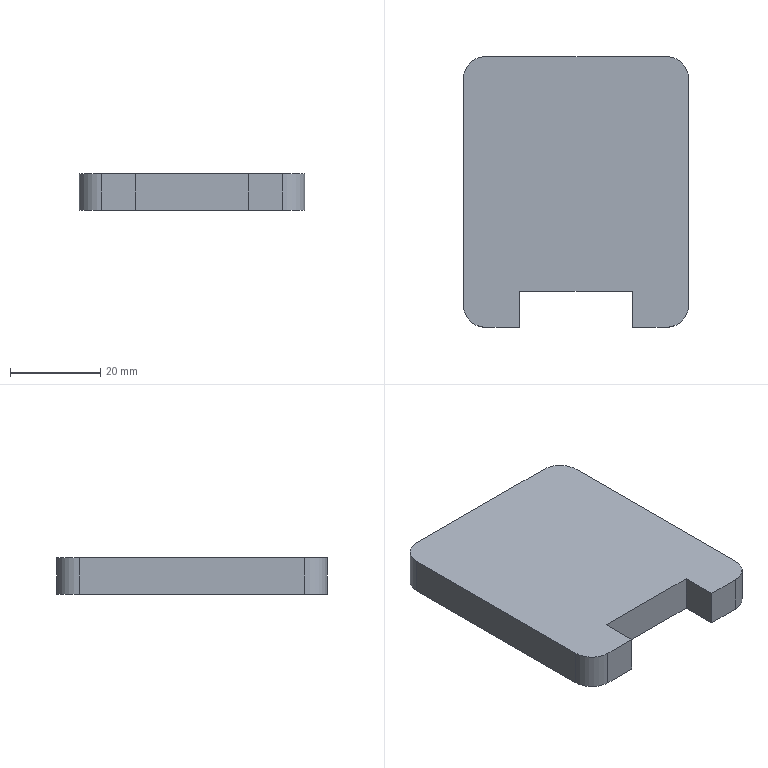Part | SolidWorks | features FlatPattern 1, SMBaseFlange 1, SheetMetal 1 | 1 solid | 14 faces | box 50 x 60 x 8 mm | volume 22228 mm3 | plane 10 | cylinder 4 | commonest cylinder face diameters 10 x4
STEP:
#1=CARTESIAN_POINT('',(-411.372,-6.5,0.));
#2=VERTEX_POINT('',#1);
#3=CARTESIAN_POINT('',(-406.372,-11.5,0.));
#4=VERTEX_POINT('',#3);
#5=CARTESIAN_POINT('',(-406.372,-6.5,0.));
#6=DIRECTION('',(0.,0.,1.));
#7=DIRECTION('',(-1.,0.,0.));
#8=AXIS2_PLACEMENT_3D('',#5,#6,#7);
#9=CIRCLE('',#8,5.);
#10=EDGE_CURVE('',#2,#4,#9,.T.);
#11=ORIENTED_EDGE('',*,*,#10,.F.);
#12=CARTESIAN_POINT('',(-411.372,-6.5,-8.));
#13=VERTEX_POINT('',#12);
#14=CARTESIAN_POINT('',(-411.372,-6.5,-8.));
#15=DIRECTION('',(0.,0.,1.));
#16=VECTOR('',#15,1000.);
#17=LINE('',#14,#16);
#18=EDGE_CURVE('',#13,#2,#17,.T.);
#19=ORIENTED_EDGE('',*,*,#18,.F.);
#20=CARTESIAN_POINT('',(-406.372,-11.5,-8.));
#21=VERTEX_POINT('',#20);
#22=CARTESIAN_POINT('',(-406.372,-6.5,-8.));
#23=DIRECTION('',(0.,0.,1.));
#24=DIRECTION('',(-1.,0.,0.));
#25=AXIS2_PLACEMENT_3D('',#22,#23,#24);
#26=CIRCLE('',#25,5.);
#27=EDGE_CURVE('',#13,#21,#26,.T.);
#28=ORIENTED_EDGE('',*,*,#27,.T.);
#29=CARTESIAN_POINT('',(-406.372,-11.5,-8.));
#30=DIRECTION('',(0.,0.,1.));
#31=VECTOR('',#30,1000.);
#32=LINE('',#29,#31);
#33=EDGE_CURVE('',#21,#4,#32,.T.);
#34=ORIENTED_EDGE('',*,*,#33,.T.);
#35=EDGE_LOOP('',(#11,#19,#28,#34));
#36=FACE_OUTER_BOUND('',#35,.T.);
#37=CARTESIAN_POINT('',(-406.372,-6.5,-8.));
#38=DIRECTION('',(0.,0.,1.));
#39=DIRECTION('',(1.,0.,0.));
#40=AXIS2_PLACEMENT_3D('',#37,#38,#39);
#41=CYLINDRICAL_SURFACE('',#40,5.);
#42=ADVANCED_FACE('',(#36),#41,.T.);
#43=CARTESIAN_POINT('',(-411.372,43.5,0.));
#44=VERTEX_POINT('',#43);
#45=CARTESIAN_POINT('',(-411.372,-6.5,0.));
#46=DIRECTION('',(0.,-1.,0.));
#47=VECTOR('',#46,1000.);
#48=LINE('',#45,#47);
#49=EDGE_CURVE('',#44,#2,#48,.T.);
#50=ORIENTED_EDGE('',*,*,#49,.F.);
#51=CARTESIAN_POINT('',(-411.372,43.5,-8.));
#52=VERTEX_POINT('',#51);
#53=CARTESIAN_POINT('',(-411.372,43.5,-8.));
#54=DIRECTION('',(0.,0.,1.));
#55=VECTOR('',#54,1000.);
#56=LINE('',#53,#55);
#57=EDGE_CURVE('',#52,#44,#56,.T.);
#58=ORIENTED_EDGE('',*,*,#57,.F.);
#59=CARTESIAN_POINT('',(-411.372,-6.5,-8.));
#60=DIRECTION('',(0.,-1.,0.));
#61=VECTOR('',#60,1000.);
#62=LINE('',#59,#61);
#63=EDGE_CURVE('',#52,#13,#62,.T.);
#64=ORIENTED_EDGE('',*,*,#63,.T.);
#65=ORIENTED_EDGE('',*,*,#18,.T.);
#66=EDGE_LOOP('',(#50,#58,#64,#65));
#67=FACE_OUTER_BOUND('',#66,.T.);
#68=CARTESIAN_POINT('',(-411.372,-6.5,-8.));
#69=DIRECTION('',(-1.,0.,0.));
#70=DIRECTION('',(0.,0.,1.));
#71=AXIS2_PLACEMENT_3D('',#68,#69,#70);
#72=PLANE('',#71);
#73=ADVANCED_FACE('',(#67),#72,.T.);
#74=CARTESIAN_POINT('',(-406.372,48.5,0.));
#75=VERTEX_POINT('',#74);
#76=CARTESIAN_POINT('',(-406.372,43.5,0.));
#77=DIRECTION('',(0.,0.,1.));
#78=DIRECTION('',(-1.,0.,0.));
#79=AXIS2_PLACEMENT_3D('',#76,#77,#78);
#80=CIRCLE('',#79,5.);
#81=EDGE_CURVE('',#75,#44,#80,.T.);
#82=ORIENTED_EDGE('',*,*,#81,.F.);
#83=CARTESIAN_POINT('',(-406.372,48.5,-8.));
#84=VERTEX_POINT('',#83);
#85=CARTESIAN_POINT('',(-406.372,48.5,-8.));
#86=DIRECTION('',(0.,0.,1.));
#87=VECTOR('',#86,1000.);
#88=LINE('',#85,#87);
#89=EDGE_CURVE('',#84,#75,#88,.T.);
#90=ORIENTED_EDGE('',*,*,#89,.F.);
#91=CARTESIAN_POINT('',(-406.372,43.5,-8.));
#92=DIRECTION('',(0.,0.,1.));
#93=DIRECTION('',(-1.,0.,0.));
#94=AXIS2_PLACEMENT_3D('',#91,#92,#93);
#95=CIRCLE('',#94,5.);
#96=EDGE_CURVE('',#84,#52,#95,.T.);
#97=ORIENTED_EDGE('',*,*,#96,.T.);
#98=ORIENTED_EDGE('',*,*,#57,.T.);
#99=EDGE_LOOP('',(#82,#90,#97,#98));
#100=FACE_OUTER_BOUND('',#99,.T.);
#101=CARTESIAN_POINT('',(-406.372,43.5,-8.));
#102=DIRECTION('',(0.,0.,1.));
#103=DIRECTION('',(1.,0.,0.));
#104=AXIS2_PLACEMENT_3D('',#101,#102,#103);
#105=CYLINDRICAL_SURFACE('',#104,5.);
#106=ADVANCED_FACE('',(#100),#105,.T.);
#107=CARTESIAN_POINT('',(-366.372,48.5,0.));
#108=VERTEX_POINT('',#107);
#109=CARTESIAN_POINT('',(-366.372,48.5,0.));
#110=DIRECTION('',(-1.,0.,0.));
#111=VECTOR('',#110,1000.);
#112=LINE('',#109,#111);
#113=EDGE_CURVE('',#108,#75,#112,.T.);
#114=ORIENTED_EDGE('',*,*,#113,.F.);
#115=CARTESIAN_POINT('',(-366.372,48.5,-8.));
#116=VERTEX_POINT('',#115);
#117=CARTESIAN_POINT('',(-366.372,48.5,-8.));
#118=DIRECTION('',(0.,0.,1.));
#119=VECTOR('',#118,1000.);
#120=LINE('',#117,#119);
#121=EDGE_CURVE('',#116,#108,#120,.T.);
#122=ORIENTED_EDGE('',*,*,#121,.F.);
#123=CARTESIAN_POINT('',(-366.372,48.5,-8.));
#124=DIRECTION('',(-1.,0.,0.));
#125=VECTOR('',#124,1000.);
#126=LINE('',#123,#125);
#127=EDGE_CURVE('',#116,#84,#126,.T.);
#128=ORIENTED_EDGE('',*,*,#127,.T.);
#129=ORIENTED_EDGE('',*,*,#89,.T.);
#130=EDGE_LOOP('',(#114,#122,#128,#129));
#131=FACE_OUTER_BOUND('',#130,.T.);
#132=CARTESIAN_POINT('',(-366.372,48.5,-8.));
#133=DIRECTION('',(0.,1.,0.));
#134=DIRECTION('',(-1.,0.,0.));
#135=AXIS2_PLACEMENT_3D('',#132,#133,#134);
#136=PLANE('',#135);
#137=ADVANCED_FACE('',(#131),#136,.T.);
#138=CARTESIAN_POINT('',(-361.372,43.5,0.));
#139=VERTEX_POINT('',#138);
#140=CARTESIAN_POINT('',(-366.372,43.5,0.));
#141=DIRECTION('',(0.,0.,1.));
#142=DIRECTION('',(1.,0.,0.));
#143=AXIS2_PLACEMENT_3D('',#140,#141,#142);
#144=CIRCLE('',#143,5.);
#145=EDGE_CURVE('',#139,#108,#144,.T.);
#146=ORIENTED_EDGE('',*,*,#145,.F.);
#147=CARTESIAN_POINT('',(-361.372,43.5,-8.));
#148=VERTEX_POINT('',#147);
#149=CARTESIAN_POINT('',(-361.372,43.5,-8.));
#150=DIRECTION('',(0.,0.,1.));
#151=VECTOR('',#150,1000.);
#152=LINE('',#149,#151);
#153=EDGE_CURVE('',#148,#139,#152,.T.);
#154=ORIENTED_EDGE('',*,*,#153,.F.);
#155=CARTESIAN_POINT('',(-366.372,43.5,-8.));
#156=DIRECTION('',(0.,0.,1.));
#157=DIRECTION('',(1.,0.,0.));
#158=AXIS2_PLACEMENT_3D('',#155,#156,#157);
#159=CIRCLE('',#158,5.);
#160=EDGE_CURVE('',#148,#116,#159,.T.);
#161=ORIENTED_EDGE('',*,*,#160,.T.);
#162=ORIENTED_EDGE('',*,*,#121,.T.);
#163=EDGE_LOOP('',(#146,#154,#161,#162));
#164=FACE_OUTER_BOUND('',#163,.T.);
#165=CARTESIAN_POINT('',(-366.372,43.5,-8.));
#166=DIRECTION('',(0.,0.,1.));
#167=DIRECTION('',(1.,0.,0.));
#168=AXIS2_PLACEMENT_3D('',#165,#166,#167);
#169=CYLINDRICAL_SURFACE('',#168,5.);
#170=ADVANCED_FACE('',(#164),#169,.T.);
#171=CARTESIAN_POINT('',(-361.372,-6.5,0.));
#172=VERTEX_POINT('',#171);
#173=CARTESIAN_POINT('',(-361.372,43.5,0.));
#174=DIRECTION('',(0.,1.,0.));
#175=VECTOR('',#174,1000.);
#176=LINE('',#173,#175);
#177=EDGE_CURVE('',#172,#139,#176,.T.);
#178=ORIENTED_EDGE('',*,*,#177,.F.);
#179=CARTESIAN_POINT('',(-361.372,-6.5,-8.));
#180=VERTEX_POINT('',#179);
#181=CARTESIAN_POINT('',(-361.372,-6.5,-8.));
#182=DIRECTION('',(0.,0.,1.));
#183=VECTOR('',#182,1000.);
#184=LINE('',#181,#183);
#185=EDGE_CURVE('',#180,#172,#184,.T.);
#186=ORIENTED_EDGE('',*,*,#185,.F.);
#187=CARTESIAN_POINT('',(-361.372,43.5,-8.));
#188=DIRECTION('',(0.,1.,0.));
#189=VECTOR('',#188,1000.);
#190=LINE('',#187,#189);
#191=EDGE_CURVE('',#180,#148,#190,.T.);
#192=ORIENTED_EDGE('',*,*,#191,.T.);
#193=ORIENTED_EDGE('',*,*,#153,.T.);
#194=EDGE_LOOP('',(#178,#186,#192,#193));
#195=FACE_OUTER_BOUND('',#194,.T.);
#196=CARTESIAN_POINT('',(-361.372,43.5,-8.));
#197=DIRECTION('',(1.,0.,0.));
#198=DIRECTION('',(0.,0.,-1.));
#199=AXIS2_PLACEMENT_3D('',#196,#197,#198);
#200=PLANE('',#199);
#201=ADVANCED_FACE('',(#195),#200,.T.);
#202=CARTESIAN_POINT('',(-366.372,-11.5,0.));
#203=VERTEX_POINT('',#202);
#204=CARTESIAN_POINT('',(-366.372,-6.5,0.));
#205=DIRECTION('',(0.,0.,1.));
#206=DIRECTION('',(-1.,0.,0.));
#207=AXIS2_PLACEMENT_3D('',#204,#205,#206);
#208=CIRCLE('',#207,5.);
#209=EDGE_CURVE('',#203,#172,#208,.T.);
#210=ORIENTED_EDGE('',*,*,#209,.F.);
#211=CARTESIAN_POINT('',(-366.372,-11.5,-8.));
#212=VERTEX_POINT('',#211);
#213=CARTESIAN_POINT('',(-366.372,-11.5,-8.));
#214=DIRECTION('',(0.,0.,1.));
#215=VECTOR('',#214,1000.);
#216=LINE('',#213,#215);
#217=EDGE_CURVE('',#212,#203,#216,.T.);
#218=ORIENTED_EDGE('',*,*,#217,.F.);
#219=CARTESIAN_POINT('',(-366.372,-6.5,-8.));
#220=DIRECTION('',(0.,0.,1.));
#221=DIRECTION('',(-1.,0.,0.));
#222=AXIS2_PLACEMENT_3D('',#219,#220,#221);
#223=CIRCLE('',#222,5.);
#224=EDGE_CURVE('',#212,#180,#223,.T.);
#225=ORIENTED_EDGE('',*,*,#224,.T.);
#226=ORIENTED_EDGE('',*,*,#185,.T.);
#227=EDGE_LOOP('',(#210,#218,#225,#226));
#228=FACE_OUTER_BOUND('',#227,.T.);
#229=CARTESIAN_POINT('',(-366.372,-6.5,-8.));
#230=DIRECTION('',(0.,0.,1.));
#231=DIRECTION('',(1.,0.,0.));
#232=AXIS2_PLACEMENT_3D('',#229,#230,#231);
#233=CYLINDRICAL_SURFACE('',#232,5.);
#234=ADVANCED_FACE('',(#228),#233,.T.);
#235=CARTESIAN_POINT('',(-373.872,-11.5,0.));
#236=VERTEX_POINT('',#235);
#237=CARTESIAN_POINT('',(-366.372,-11.5,0.));
#238=DIRECTION('',(1.,0.,0.));
#239=VECTOR('',#238,1000.);
#240=LINE('',#237,#239);
#241=EDGE_CURVE('',#236,#203,#240,.T.);
#242=ORIENTED_EDGE('',*,*,#241,.F.);
#243=CARTESIAN_POINT('',(-373.872,-11.5,-8.));
#244=VERTEX_POINT('',#243);
#245=CARTESIAN_POINT('',(-373.872,-11.5,-8.));
#246=DIRECTION('',(0.,0.,1.));
#247=VECTOR('',#246,1000.);
#248=LINE('',#245,#247);
#249=EDGE_CURVE('',#244,#236,#248,.T.);
#250=ORIENTED_EDGE('',*,*,#249,.F.);
#251=CARTESIAN_POINT('',(-366.372,-11.5,-8.));
#252=DIRECTION('',(1.,0.,0.));
#253=VECTOR('',#252,1000.);
#254=LINE('',#251,#253);
#255=EDGE_CURVE('',#244,#212,#254,.T.);
#256=ORIENTED_EDGE('',*,*,#255,.T.);
#257=ORIENTED_EDGE('',*,*,#217,.T.);
#258=EDGE_LOOP('',(#242,#250,#256,#257));
#259=FACE_OUTER_BOUND('',#258,.T.);
#260=CARTESIAN_POINT('',(-366.372,-11.5,-8.));
#261=DIRECTION('',(0.,-1.,0.));
#262=DIRECTION('',(1.,0.,0.));
#263=AXIS2_PLACEMENT_3D('',#260,#261,#262);
#264=PLANE('',#263);
#265=ADVANCED_FACE('',(#259),#264,.T.);
#266=CARTESIAN_POINT('',(-373.872,-3.5,0.));
#267=VERTEX_POINT('',#266);
#268=CARTESIAN_POINT('',(-373.872,-11.5,0.));
#269=DIRECTION('',(0.,-1.,0.));
#270=VECTOR('',#269,1000.);
#271=LINE('',#268,#270);
#272=EDGE_CURVE('',#267,#236,#271,.T.);
#273=ORIENTED_EDGE('',*,*,#272,.F.);
#274=CARTESIAN_POINT('',(-373.872,-3.5,-8.));
#275=VERTEX_POINT('',#274);
#276=CARTESIAN_POINT('',(-373.872,-3.5,-8.));
#277=DIRECTION('',(0.,0.,1.));
#278=VECTOR('',#277,1000.);
#279=LINE('',#276,#278);
#280=EDGE_CURVE('',#275,#267,#279,.T.);
#281=ORIENTED_EDGE('',*,*,#280,.F.);
#282=CARTESIAN_POINT('',(-373.872,-11.5,-8.));
#283=DIRECTION('',(0.,-1.,0.));
#284=VECTOR('',#283,1000.);
#285=LINE('',#282,#284);
#286=EDGE_CURVE('',#275,#244,#285,.T.);
#287=ORIENTED_EDGE('',*,*,#286,.T.);
#288=ORIENTED_EDGE('',*,*,#249,.T.);
#289=EDGE_LOOP('',(#273,#281,#287,#288));
#290=FACE_OUTER_BOUND('',#289,.T.);
#291=CARTESIAN_POINT('',(-373.872,-11.5,-8.));
#292=DIRECTION('',(-1.,0.,0.));
#293=DIRECTION('',(0.,0.,1.));
#294=AXIS2_PLACEMENT_3D('',#291,#292,#293);
#295=PLANE('',#294);
#296=ADVANCED_FACE('',(#290),#295,.T.);
#297=CARTESIAN_POINT('',(-398.872,-3.5,0.));
#298=VERTEX_POINT('',#297);
#299=CARTESIAN_POINT('',(-373.872,-3.5,0.));
#300=DIRECTION('',(1.,0.,0.));
#301=VECTOR('',#300,1000.);
#302=LINE('',#299,#301);
#303=EDGE_CURVE('',#298,#267,#302,.T.);
#304=ORIENTED_EDGE('',*,*,#303,.F.);
#305=CARTESIAN_POINT('',(-398.872,-3.5,-8.));
#306=VERTEX_POINT('',#305);
#307=CARTESIAN_POINT('',(-398.872,-3.5,-8.));
#308=DIRECTION('',(0.,0.,1.));
#309=VECTOR('',#308,1000.);
#310=LINE('',#307,#309);
#311=EDGE_CURVE('',#306,#298,#310,.T.);
#312=ORIENTED_EDGE('',*,*,#311,.F.);
#313=CARTESIAN_POINT('',(-373.872,-3.5,-8.));
#314=DIRECTION('',(1.,0.,0.));
#315=VECTOR('',#314,1000.);
#316=LINE('',#313,#315);
#317=EDGE_CURVE('',#306,#275,#316,.T.);
#318=ORIENTED_EDGE('',*,*,#317,.T.);
#319=ORIENTED_EDGE('',*,*,#280,.T.);
#320=EDGE_LOOP('',(#304,#312,#318,#319));
#321=FACE_OUTER_BOUND('',#320,.T.);
#322=CARTESIAN_POINT('',(-373.872,-3.5,-8.));
#323=DIRECTION('',(0.,-1.,0.));
#324=DIRECTION('',(0.,0.,-1.));
#325=AXIS2_PLACEMENT_3D('',#322,#323,#324);
#326=PLANE('',#325);
#327=ADVANCED_FACE('',(#321),#326,.T.);
#328=CARTESIAN_POINT('',(-398.872,-11.5,0.));
#329=VERTEX_POINT('',#328);
#330=CARTESIAN_POINT('',(-398.872,-11.5,0.));
#331=DIRECTION('',(0.,1.,0.));
#332=VECTOR('',#331,1000.);
#333=LINE('',#330,#332);
#334=EDGE_CURVE('',#329,#298,#333,.T.);
#335=ORIENTED_EDGE('',*,*,#334,.F.);
#336=CARTESIAN_POINT('',(-398.872,-11.5,-8.));
#337=VERTEX_POINT('',#336);
#338=CARTESIAN_POINT('',(-398.872,-11.5,-8.));
#339=DIRECTION('',(0.,0.,1.));
#340=VECTOR('',#339,1000.);
#341=LINE('',#338,#340);
#342=EDGE_CURVE('',#337,#329,#341,.T.);
#343=ORIENTED_EDGE('',*,*,#342,.F.);
#344=CARTESIAN_POINT('',(-398.872,-11.5,-8.));
#345=DIRECTION('',(0.,1.,0.));
#346=VECTOR('',#345,1000.);
#347=LINE('',#344,#346);
#348=EDGE_CURVE('',#337,#306,#347,.T.);
#349=ORIENTED_EDGE('',*,*,#348,.T.);
#350=ORIENTED_EDGE('',*,*,#311,.T.);
#351=EDGE_LOOP('',(#335,#343,#349,#350));
#352=FACE_OUTER_BOUND('',#351,.T.);
#353=CARTESIAN_POINT('',(-398.872,-11.5,-8.));
#354=DIRECTION('',(1.,0.,0.));
#355=DIRECTION('',(0.,0.,-1.));
#356=AXIS2_PLACEMENT_3D('',#353,#354,#355);
#357=PLANE('',#356);
#358=ADVANCED_FACE('',(#352),#357,.T.);
#359=CARTESIAN_POINT('',(-398.872,-11.5,0.));
#360=DIRECTION('',(1.,0.,0.));
#361=VECTOR('',#360,1000.);
#362=LINE('',#359,#361);
#363=EDGE_CURVE('',#4,#329,#362,.T.);
#364=ORIENTED_EDGE('',*,*,#363,.F.);
#365=ORIENTED_EDGE('',*,*,#33,.F.);
#366=CARTESIAN_POINT('',(-398.872,-11.5,-8.));
#367=DIRECTION('',(1.,0.,0.));
#368=VECTOR('',#367,1000.);
#369=LINE('',#366,#368);
#370=EDGE_CURVE('',#21,#337,#369,.T.);
#371=ORIENTED_EDGE('',*,*,#370,.T.);
#372=ORIENTED_EDGE('',*,*,#342,.T.);
#373=EDGE_LOOP('',(#364,#365,#371,#372));
#374=FACE_OUTER_BOUND('',#373,.T.);
#375=CARTESIAN_POINT('',(-398.872,-11.5,-8.));
#376=DIRECTION('',(0.,-1.,0.));
#377=DIRECTION('',(1.,0.,0.));
#378=AXIS2_PLACEMENT_3D('',#375,#376,#377);
#379=PLANE('',#378);
#380=ADVANCED_FACE('',(#374),#379,.T.);
#381=ORIENTED_EDGE('',*,*,#27,.F.);
#382=ORIENTED_EDGE('',*,*,#63,.F.);
#383=ORIENTED_EDGE('',*,*,#96,.F.);
#384=ORIENTED_EDGE('',*,*,#127,.F.);
#385=ORIENTED_EDGE('',*,*,#160,.F.);
#386=ORIENTED_EDGE('',*,*,#191,.F.);
#387=ORIENTED_EDGE('',*,*,#224,.F.);
#388=ORIENTED_EDGE('',*,*,#255,.F.);
#389=ORIENTED_EDGE('',*,*,#286,.F.);
#390=ORIENTED_EDGE('',*,*,#317,.F.);
#391=ORIENTED_EDGE('',*,*,#348,.F.);
#392=ORIENTED_EDGE('',*,*,#370,.F.);
#393=EDGE_LOOP('',(#381,#382,#383,#384,#385,#386,#387,#388,#389,#390,#391,#392));
#394=FACE_OUTER_BOUND('',#393,.T.);
#395=CARTESIAN_POINT('',(-406.372,-6.5,-8.));
#396=DIRECTION('',(0.,0.,-1.));
#397=DIRECTION('',(-1.,0.,0.));
#398=AXIS2_PLACEMENT_3D('',#395,#396,#397);
#399=PLANE('',#398);
#400=ADVANCED_FACE('',(#394),#399,.T.);
#401=ORIENTED_EDGE('',*,*,#10,.T.);
#402=ORIENTED_EDGE('',*,*,#363,.T.);
#403=ORIENTED_EDGE('',*,*,#334,.T.);
#404=ORIENTED_EDGE('',*,*,#303,.T.);
#405=ORIENTED_EDGE('',*,*,#272,.T.);
#406=ORIENTED_EDGE('',*,*,#241,.T.);
#407=ORIENTED_EDGE('',*,*,#209,.T.);
#408=ORIENTED_EDGE('',*,*,#177,.T.);
#409=ORIENTED_EDGE('',*,*,#145,.T.);
#410=ORIENTED_EDGE('',*,*,#113,.T.);
#411=ORIENTED_EDGE('',*,*,#81,.T.);
#412=ORIENTED_EDGE('',*,*,#49,.T.);
#413=EDGE_LOOP('',(#401,#402,#403,#404,#405,#406,#407,#408,#409,#410,#411,#412));
#414=FACE_OUTER_BOUND('',#413,.T.);
#415=CARTESIAN_POINT('',(-406.372,-6.5,0.));
#416=DIRECTION('',(0.,0.,-1.));
#417=DIRECTION('',(-1.,0.,0.));
#418=AXIS2_PLACEMENT_3D('',#415,#416,#417);
#419=PLANE('',#418);
#420=ADVANCED_FACE('',(#414),#419,.F.);
#421=CLOSED_SHELL('',(#42,#73,#106,#137,#170,#201,#234,#265,#296,#327,#358,#380,#400,#420));
#422=MANIFOLD_SOLID_BREP('',#421);
#423=CARTESIAN_POINT('',(0.,0.,0.));
#424=DIRECTION('',(0.,0.,1.));
#425=DIRECTION('',(1.,0.,0.));
#426=AXIS2_PLACEMENT_3D('',#423,#424,#425);
#427=(LENGTH_UNIT()NAMED_UNIT(*)SI_UNIT(.MILLI.,.METRE.));
#428=UNCERTAINTY_MEASURE_WITH_UNIT(LENGTH_MEASURE(0.00001),#427,'','');
#429=(NAMED_UNIT(*)PLANE_ANGLE_UNIT()SI_UNIT($,.RADIAN.));
#430=(NAMED_UNIT(*)SI_UNIT($,.STERADIAN.)SOLID_ANGLE_UNIT());
#431=(GEOMETRIC_REPRESENTATION_CONTEXT(3)GLOBAL_UNCERTAINTY_ASSIGNED_CONTEXT((#428))GLOBAL_UNIT_ASSIGNED_CONTEXT((#427,#429,#430))REPRESENTATION_CONTEXT('',''));
#432=ADVANCED_BREP_SHAPE_REPRESENTATION('',(#422,#426),#431);